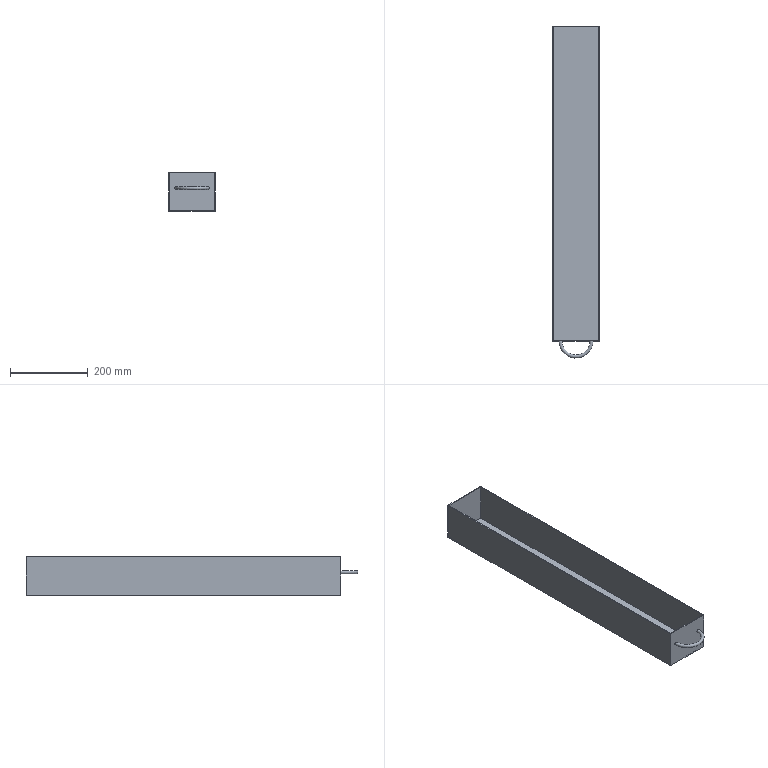Part | NX | features solid 2 | 1 solid | 12 faces | box 120 x 854 x 100 mm | volume 563709 mm3 | plane 11 | torus 1
STEP:
#1=CARTESIAN_POINT('',(720.,-805.,-386.));
#2=VERTEX_POINT('',#1);
#3=CARTESIAN_POINT('',(720.,-805.,-390.));
#4=DIRECTION('',(0.,-1.,0.));
#5=DIRECTION('',(0.,0.,1.));
#6=AXIS2_PLACEMENT_3D('',#3,#4,#5);
#7=CIRCLE('',#6,4.);
#8=EDGE_CURVE('',#2,#2,#7,.F.);
#9=ORIENTED_EDGE('',*,*,#8,.T.);
#10=EDGE_LOOP('',(#9));
#11=FACE_BOUND('',#10,.T.);
#12=CARTESIAN_POINT('',(740.,-805.,-450.));
#13=VERTEX_POINT('',#12);
#14=CARTESIAN_POINT('',(620.,-805.,-450.));
#15=VERTEX_POINT('',#14);
#16=CARTESIAN_POINT('',(1300.,-805.,-450.));
#17=DIRECTION('',(-1.,0.,0.));
#18=VECTOR('',#17,1000.);
#19=LINE('',#16,#18);
#20=EDGE_CURVE('',#13,#15,#19,.T.);
#21=ORIENTED_EDGE('',*,*,#20,.F.);
#22=CARTESIAN_POINT('',(740.,-805.,-350.));
#23=VERTEX_POINT('',#22);
#24=CARTESIAN_POINT('',(740.,-805.,-448.));
#25=DIRECTION('',(0.,0.,-1.));
#26=VECTOR('',#25,1000.);
#27=LINE('',#24,#26);
#28=EDGE_CURVE('',#23,#13,#27,.T.);
#29=ORIENTED_EDGE('',*,*,#28,.F.);
#30=CARTESIAN_POINT('',(620.,-805.,-350.));
#31=VERTEX_POINT('',#30);
#32=CARTESIAN_POINT('',(1300.,-805.,-350.));
#33=DIRECTION('',(-1.,0.,0.));
#34=VECTOR('',#33,1000.);
#35=LINE('',#32,#34);
#36=EDGE_CURVE('',#23,#31,#35,.T.);
#37=ORIENTED_EDGE('',*,*,#36,.T.);
#38=CARTESIAN_POINT('',(620.,-805.,-448.));
#39=DIRECTION('',(0.,0.,-1.));
#40=VECTOR('',#39,1000.);
#41=LINE('',#38,#40);
#42=EDGE_CURVE('',#31,#15,#41,.T.);
#43=ORIENTED_EDGE('',*,*,#42,.T.);
#44=EDGE_LOOP('',(#21,#29,#37,#43));
#45=FACE_BOUND('',#44,.T.);
#46=CARTESIAN_POINT('',(640.,-805.,-386.));
#47=VERTEX_POINT('',#46);
#48=CARTESIAN_POINT('',(640.,-805.,-390.));
#49=DIRECTION('',(0.,-1.,0.));
#50=DIRECTION('',(0.,0.,1.));
#51=AXIS2_PLACEMENT_3D('',#48,#49,#50);
#52=CIRCLE('',#51,4.);
#53=EDGE_CURVE('',#47,#47,#52,.F.);
#54=ORIENTED_EDGE('',*,*,#53,.T.);
#55=EDGE_LOOP('',(#54));
#56=FACE_BOUND('',#55,.T.);
#57=CARTESIAN_POINT('',(1300.,-805.,-448.));
#58=DIRECTION('',(0.,1.,0.));
#59=DIRECTION('',(0.,0.,1.));
#60=AXIS2_PLACEMENT_3D('',#57,#58,#59);
#61=PLANE('',#60);
#62=ADVANCED_FACE('',(#11,#45,#56),#61,.F.);
#63=CARTESIAN_POINT('',(740.,5.,-350.));
#64=VERTEX_POINT('',#63);
#65=CARTESIAN_POINT('',(740.,-965.,-350.));
#66=DIRECTION('',(0.,1.,0.));
#67=VECTOR('',#66,1000.);
#68=LINE('',#65,#67);
#69=EDGE_CURVE('',#23,#64,#68,.T.);
#70=ORIENTED_EDGE('',*,*,#69,.T.);
#71=CARTESIAN_POINT('',(620.,5.,-350.));
#72=VERTEX_POINT('',#71);
#73=CARTESIAN_POINT('',(1300.,5.,-350.));
#74=DIRECTION('',(-1.,0.,0.));
#75=VECTOR('',#74,1000.);
#76=LINE('',#73,#75);
#77=EDGE_CURVE('',#64,#72,#76,.T.);
#78=ORIENTED_EDGE('',*,*,#77,.T.);
#79=CARTESIAN_POINT('',(620.,-965.,-350.));
#80=DIRECTION('',(0.,1.,0.));
#81=VECTOR('',#80,1000.);
#82=LINE('',#79,#81);
#83=EDGE_CURVE('',#31,#72,#82,.T.);
#84=ORIENTED_EDGE('',*,*,#83,.F.);
#85=ORIENTED_EDGE('',*,*,#36,.F.);
#86=EDGE_LOOP('',(#70,#78,#84,#85));
#87=FACE_BOUND('',#86,.T.);
#88=CARTESIAN_POINT('',(738.,-803.,-350.));
#89=VERTEX_POINT('',#88);
#90=CARTESIAN_POINT('',(622.,-803.,-350.));
#91=VERTEX_POINT('',#90);
#92=CARTESIAN_POINT('',(1300.,-803.,-350.));
#93=DIRECTION('',(-1.,0.,0.));
#94=VECTOR('',#93,1000.);
#95=LINE('',#92,#94);
#96=EDGE_CURVE('',#89,#91,#95,.T.);
#97=ORIENTED_EDGE('',*,*,#96,.T.);
#98=CARTESIAN_POINT('',(622.,3.,-350.));
#99=VERTEX_POINT('',#98);
#100=CARTESIAN_POINT('',(622.,-965.,-350.));
#101=DIRECTION('',(0.,1.,0.));
#102=VECTOR('',#101,1000.);
#103=LINE('',#100,#102);
#104=EDGE_CURVE('',#91,#99,#103,.T.);
#105=ORIENTED_EDGE('',*,*,#104,.T.);
#106=CARTESIAN_POINT('',(738.,3.,-350.));
#107=VERTEX_POINT('',#106);
#108=CARTESIAN_POINT('',(1300.,3.,-350.));
#109=DIRECTION('',(-1.,0.,0.));
#110=VECTOR('',#109,1000.);
#111=LINE('',#108,#110);
#112=EDGE_CURVE('',#107,#99,#111,.T.);
#113=ORIENTED_EDGE('',*,*,#112,.F.);
#114=CARTESIAN_POINT('',(738.,-965.,-350.));
#115=DIRECTION('',(0.,1.,0.));
#116=VECTOR('',#115,1000.);
#117=LINE('',#114,#116);
#118=EDGE_CURVE('',#89,#107,#117,.T.);
#119=ORIENTED_EDGE('',*,*,#118,.F.);
#120=EDGE_LOOP('',(#97,#105,#113,#119));
#121=FACE_BOUND('',#120,.T.);
#122=CARTESIAN_POINT('',(990.,-682.5,-350.));
#123=DIRECTION('',(0.,0.,1.));
#124=DIRECTION('',(-1.,0.,0.));
#125=AXIS2_PLACEMENT_3D('',#122,#123,#124);
#126=PLANE('',#125);
#127=ADVANCED_FACE('',(#87,#121),#126,.T.);
#128=CARTESIAN_POINT('',(740.,5.,-450.));
#129=VERTEX_POINT('',#128);
#130=CARTESIAN_POINT('',(740.,-965.,-450.));
#131=DIRECTION('',(0.,1.,0.));
#132=VECTOR('',#131,1000.);
#133=LINE('',#130,#132);
#134=EDGE_CURVE('',#13,#129,#133,.T.);
#135=ORIENTED_EDGE('',*,*,#134,.T.);
#136=CARTESIAN_POINT('',(740.,5.,-448.));
#137=DIRECTION('',(0.,0.,-1.));
#138=VECTOR('',#137,1000.);
#139=LINE('',#136,#138);
#140=EDGE_CURVE('',#64,#129,#139,.T.);
#141=ORIENTED_EDGE('',*,*,#140,.F.);
#142=ORIENTED_EDGE('',*,*,#69,.F.);
#143=ORIENTED_EDGE('',*,*,#28,.T.);
#144=EDGE_LOOP('',(#135,#141,#142,#143));
#145=FACE_BOUND('',#144,.T.);
#146=CARTESIAN_POINT('',(740.,-965.,-448.));
#147=DIRECTION('',(1.,0.,0.));
#148=DIRECTION('',(0.,0.,1.));
#149=AXIS2_PLACEMENT_3D('',#146,#147,#148);
#150=PLANE('',#149);
#151=ADVANCED_FACE('',(#145),#150,.T.);
#152=CARTESIAN_POINT('',(620.,5.,-450.));
#153=VERTEX_POINT('',#152);
#154=CARTESIAN_POINT('',(620.,-965.,-450.));
#155=DIRECTION('',(0.,1.,0.));
#156=VECTOR('',#155,1000.);
#157=LINE('',#154,#156);
#158=EDGE_CURVE('',#15,#153,#157,.T.);
#159=ORIENTED_EDGE('',*,*,#158,.F.);
#160=ORIENTED_EDGE('',*,*,#42,.F.);
#161=ORIENTED_EDGE('',*,*,#83,.T.);
#162=CARTESIAN_POINT('',(620.,5.,-448.));
#163=DIRECTION('',(0.,0.,-1.));
#164=VECTOR('',#163,1000.);
#165=LINE('',#162,#164);
#166=EDGE_CURVE('',#72,#153,#165,.T.);
#167=ORIENTED_EDGE('',*,*,#166,.T.);
#168=EDGE_LOOP('',(#159,#160,#161,#167));
#169=FACE_BOUND('',#168,.T.);
#170=CARTESIAN_POINT('',(620.,-965.,-448.));
#171=DIRECTION('',(1.,0.,0.));
#172=DIRECTION('',(0.,0.,1.));
#173=AXIS2_PLACEMENT_3D('',#170,#171,#172);
#174=PLANE('',#173);
#175=ADVANCED_FACE('',(#169),#174,.F.);
#176=CARTESIAN_POINT('',(1300.,5.,-450.));
#177=DIRECTION('',(-1.,0.,0.));
#178=VECTOR('',#177,1000.);
#179=LINE('',#176,#178);
#180=EDGE_CURVE('',#129,#153,#179,.T.);
#181=ORIENTED_EDGE('',*,*,#180,.T.);
#182=ORIENTED_EDGE('',*,*,#166,.F.);
#183=ORIENTED_EDGE('',*,*,#77,.F.);
#184=ORIENTED_EDGE('',*,*,#140,.T.);
#185=EDGE_LOOP('',(#181,#182,#183,#184));
#186=FACE_BOUND('',#185,.T.);
#187=CARTESIAN_POINT('',(1300.,5.,-448.));
#188=DIRECTION('',(0.,1.,0.));
#189=DIRECTION('',(1.,0.,0.));
#190=AXIS2_PLACEMENT_3D('',#187,#188,#189);
#191=PLANE('',#190);
#192=ADVANCED_FACE('',(#186),#191,.T.);
#193=ORIENTED_EDGE('',*,*,#134,.F.);
#194=ORIENTED_EDGE('',*,*,#20,.T.);
#195=ORIENTED_EDGE('',*,*,#158,.T.);
#196=ORIENTED_EDGE('',*,*,#180,.F.);
#197=EDGE_LOOP('',(#193,#194,#195,#196));
#198=FACE_BOUND('',#197,.T.);
#199=CARTESIAN_POINT('',(990.,-682.5,-450.));
#200=DIRECTION('',(0.,0.,1.));
#201=DIRECTION('',(-1.,0.,0.));
#202=AXIS2_PLACEMENT_3D('',#199,#200,#201);
#203=PLANE('',#202);
#204=ADVANCED_FACE('',(#198),#203,.F.);
#205=CARTESIAN_POINT('',(738.,-803.,-448.));
#206=VERTEX_POINT('',#205);
#207=CARTESIAN_POINT('',(738.,3.,-448.));
#208=VERTEX_POINT('',#207);
#209=CARTESIAN_POINT('',(738.,-965.,-448.));
#210=DIRECTION('',(0.,1.,0.));
#211=VECTOR('',#210,1000.);
#212=LINE('',#209,#211);
#213=EDGE_CURVE('',#206,#208,#212,.T.);
#214=ORIENTED_EDGE('',*,*,#213,.F.);
#215=CARTESIAN_POINT('',(738.,-803.,-448.));
#216=DIRECTION('',(0.,0.,-1.));
#217=VECTOR('',#216,1000.);
#218=LINE('',#215,#217);
#219=EDGE_CURVE('',#89,#206,#218,.T.);
#220=ORIENTED_EDGE('',*,*,#219,.F.);
#221=ORIENTED_EDGE('',*,*,#118,.T.);
#222=CARTESIAN_POINT('',(738.,3.,-448.));
#223=DIRECTION('',(0.,0.,-1.));
#224=VECTOR('',#223,1000.);
#225=LINE('',#222,#224);
#226=EDGE_CURVE('',#107,#208,#225,.T.);
#227=ORIENTED_EDGE('',*,*,#226,.T.);
#228=EDGE_LOOP('',(#214,#220,#221,#227));
#229=FACE_BOUND('',#228,.T.);
#230=CARTESIAN_POINT('',(738.,-965.,-448.));
#231=DIRECTION('',(1.,0.,0.));
#232=DIRECTION('',(0.,0.,1.));
#233=AXIS2_PLACEMENT_3D('',#230,#231,#232);
#234=PLANE('',#233);
#235=ADVANCED_FACE('',(#229),#234,.F.);
#236=CARTESIAN_POINT('',(622.,-803.,-448.));
#237=VERTEX_POINT('',#236);
#238=CARTESIAN_POINT('',(1300.,-803.,-448.));
#239=DIRECTION('',(-1.,0.,0.));
#240=VECTOR('',#239,1000.);
#241=LINE('',#238,#240);
#242=EDGE_CURVE('',#206,#237,#241,.T.);
#243=ORIENTED_EDGE('',*,*,#242,.T.);
#244=CARTESIAN_POINT('',(622.,-803.,-448.));
#245=DIRECTION('',(0.,0.,-1.));
#246=VECTOR('',#245,1000.);
#247=LINE('',#244,#246);
#248=EDGE_CURVE('',#91,#237,#247,.T.);
#249=ORIENTED_EDGE('',*,*,#248,.F.);
#250=ORIENTED_EDGE('',*,*,#96,.F.);
#251=ORIENTED_EDGE('',*,*,#219,.T.);
#252=EDGE_LOOP('',(#243,#249,#250,#251));
#253=FACE_BOUND('',#252,.T.);
#254=CARTESIAN_POINT('',(1300.,-803.,-448.));
#255=DIRECTION('',(0.,1.,0.));
#256=DIRECTION('',(0.,0.,1.));
#257=AXIS2_PLACEMENT_3D('',#254,#255,#256);
#258=PLANE('',#257);
#259=ADVANCED_FACE('',(#253),#258,.T.);
#260=CARTESIAN_POINT('',(622.,3.,-448.));
#261=VERTEX_POINT('',#260);
#262=CARTESIAN_POINT('',(622.,-965.,-448.));
#263=DIRECTION('',(0.,1.,0.));
#264=VECTOR('',#263,1000.);
#265=LINE('',#262,#264);
#266=EDGE_CURVE('',#237,#261,#265,.T.);
#267=ORIENTED_EDGE('',*,*,#266,.T.);
#268=CARTESIAN_POINT('',(622.,3.,-448.));
#269=DIRECTION('',(0.,0.,-1.));
#270=VECTOR('',#269,1000.);
#271=LINE('',#268,#270);
#272=EDGE_CURVE('',#99,#261,#271,.T.);
#273=ORIENTED_EDGE('',*,*,#272,.F.);
#274=ORIENTED_EDGE('',*,*,#104,.F.);
#275=ORIENTED_EDGE('',*,*,#248,.T.);
#276=EDGE_LOOP('',(#267,#273,#274,#275));
#277=FACE_BOUND('',#276,.T.);
#278=CARTESIAN_POINT('',(622.,-965.,-448.));
#279=DIRECTION('',(1.,0.,0.));
#280=DIRECTION('',(0.,0.,1.));
#281=AXIS2_PLACEMENT_3D('',#278,#279,#280);
#282=PLANE('',#281);
#283=ADVANCED_FACE('',(#277),#282,.T.);
#284=CARTESIAN_POINT('',(1300.,3.,-448.));
#285=DIRECTION('',(-1.,0.,0.));
#286=VECTOR('',#285,1000.);
#287=LINE('',#284,#286);
#288=EDGE_CURVE('',#208,#261,#287,.T.);
#289=ORIENTED_EDGE('',*,*,#288,.F.);
#290=ORIENTED_EDGE('',*,*,#226,.F.);
#291=ORIENTED_EDGE('',*,*,#112,.T.);
#292=ORIENTED_EDGE('',*,*,#272,.T.);
#293=EDGE_LOOP('',(#289,#290,#291,#292));
#294=FACE_BOUND('',#293,.T.);
#295=CARTESIAN_POINT('',(1300.,3.,-448.));
#296=DIRECTION('',(0.,1.,0.));
#297=DIRECTION('',(1.,0.,0.));
#298=AXIS2_PLACEMENT_3D('',#295,#296,#297);
#299=PLANE('',#298);
#300=ADVANCED_FACE('',(#294),#299,.F.);
#301=ORIENTED_EDGE('',*,*,#213,.T.);
#302=ORIENTED_EDGE('',*,*,#288,.T.);
#303=ORIENTED_EDGE('',*,*,#266,.F.);
#304=ORIENTED_EDGE('',*,*,#242,.F.);
#305=EDGE_LOOP('',(#301,#302,#303,#304));
#306=FACE_BOUND('',#305,.T.);
#307=CARTESIAN_POINT('',(990.,-682.5,-448.));
#308=DIRECTION('',(0.,0.,1.));
#309=DIRECTION('',(-1.,0.,0.));
#310=AXIS2_PLACEMENT_3D('',#307,#308,#309);
#311=PLANE('',#310);
#312=ADVANCED_FACE('',(#306),#311,.T.);
#313=ORIENTED_EDGE('',*,*,#8,.F.);
#314=EDGE_LOOP('',(#313));
#315=FACE_BOUND('',#314,.T.);
#316=ORIENTED_EDGE('',*,*,#53,.F.);
#317=EDGE_LOOP('',(#316));
#318=FACE_BOUND('',#317,.T.);
#319=CARTESIAN_POINT('',(680.,-805.,-390.));
#320=DIRECTION('',(0.,0.,-1.));
#321=DIRECTION('',(1.,0.,0.));
#322=AXIS2_PLACEMENT_3D('',#319,#320,#321);
#323=TOROIDAL_SURFACE('',#322,40.,4.);
#324=ADVANCED_FACE('',(#315,#318),#323,.T.);
#325=CLOSED_SHELL('',(#62,#127,#151,#175,#192,#204,#235,#259,#283,#300,#312,#324));
#326=MANIFOLD_SOLID_BREP('',#325);
#327=(LENGTH_UNIT()NAMED_UNIT(*)SI_UNIT(.MILLI.,.METRE.));
#328=UNCERTAINTY_MEASURE_WITH_UNIT(LENGTH_MEASURE(0.00001),#327,'','');
#329=(NAMED_UNIT(*)PLANE_ANGLE_UNIT()SI_UNIT($,.RADIAN.));
#330=(NAMED_UNIT(*)SI_UNIT($,.STERADIAN.)SOLID_ANGLE_UNIT());
#331=(GEOMETRIC_REPRESENTATION_CONTEXT(3)GLOBAL_UNCERTAINTY_ASSIGNED_CONTEXT((#328))GLOBAL_UNIT_ASSIGNED_CONTEXT((#327,#329,#330))REPRESENTATION_CONTEXT('',''));
#332=ADVANCED_BREP_SHAPE_REPRESENTATION('',(#326),#331);